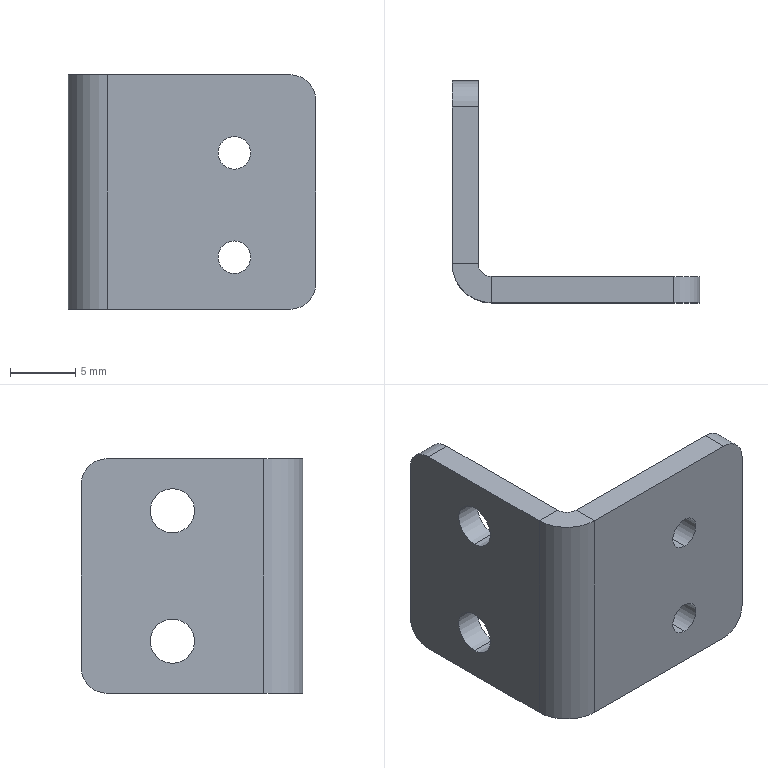Part | NX | features BREP 1 | 1 solid | 26 faces | box 19 x 17 x 18 mm | volume 1130 mm3 | cylinder 14 | plane 12 | commonest cylinder face diameters 2.5 x4 3.4 x4 4 x4 2 x1 6 x1
STEP:
#1=CARTESIAN_POINT('',(-2.,8.,6.7));
#2=VERTEX_POINT('',#1);
#3=CARTESIAN_POINT('',(0.,8.,6.7));
#4=VERTEX_POINT('',#3);
#5=CARTESIAN_POINT('',(0.,8.,6.7));
#6=DIRECTION('',(1.,0.,0.));
#7=VECTOR('',#6,1000.);
#8=LINE('',#5,#7);
#9=EDGE_CURVE('',#2,#4,#8,.T.);
#10=ORIENTED_EDGE('',*,*,#9,.F.);
#11=CARTESIAN_POINT('',(-2.,8.,3.3));
#12=VERTEX_POINT('',#11);
#13=CARTESIAN_POINT('',(-2.,8.,5.));
#14=DIRECTION('',(1.,0.,0.));
#15=DIRECTION('',(0.,0.,-1.));
#16=AXIS2_PLACEMENT_3D('',#13,#14,#15);
#17=CIRCLE('',#16,1.7);
#18=EDGE_CURVE('',#12,#2,#17,.T.);
#19=ORIENTED_EDGE('',*,*,#18,.F.);
#20=CARTESIAN_POINT('',(0.,8.,3.3));
#21=VERTEX_POINT('',#20);
#22=CARTESIAN_POINT('',(0.,8.,3.3));
#23=DIRECTION('',(1.,0.,0.));
#24=VECTOR('',#23,1000.);
#25=LINE('',#22,#24);
#26=EDGE_CURVE('',#12,#21,#25,.T.);
#27=ORIENTED_EDGE('',*,*,#26,.T.);
#28=CARTESIAN_POINT('',(0.,8.,5.));
#29=DIRECTION('',(1.,0.,0.));
#30=DIRECTION('',(0.,0.,-1.));
#31=AXIS2_PLACEMENT_3D('',#28,#29,#30);
#32=CIRCLE('',#31,1.7);
#33=EDGE_CURVE('',#21,#4,#32,.T.);
#34=ORIENTED_EDGE('',*,*,#33,.T.);
#35=EDGE_LOOP('',(#10,#19,#27,#34));
#36=FACE_BOUND('',#35,.T.);
#37=CARTESIAN_POINT('',(0.,8.,5.));
#38=DIRECTION('',(1.,0.,0.));
#39=DIRECTION('',(0.,0.,-1.));
#40=AXIS2_PLACEMENT_3D('',#37,#38,#39);
#41=CYLINDRICAL_SURFACE('',#40,1.7);
#42=ADVANCED_FACE('',(#36),#41,.F.);
#43=CARTESIAN_POINT('',(-2.,8.,-3.3));
#44=VERTEX_POINT('',#43);
#45=CARTESIAN_POINT('',(0.,8.,-3.3));
#46=VERTEX_POINT('',#45);
#47=CARTESIAN_POINT('',(0.,8.,-3.3));
#48=DIRECTION('',(1.,0.,0.));
#49=VECTOR('',#48,1000.);
#50=LINE('',#47,#49);
#51=EDGE_CURVE('',#44,#46,#50,.T.);
#52=ORIENTED_EDGE('',*,*,#51,.F.);
#53=CARTESIAN_POINT('',(-2.,8.,-6.7));
#54=VERTEX_POINT('',#53);
#55=CARTESIAN_POINT('',(-2.,8.,-5.));
#56=DIRECTION('',(1.,0.,0.));
#57=DIRECTION('',(0.,0.,-1.));
#58=AXIS2_PLACEMENT_3D('',#55,#56,#57);
#59=CIRCLE('',#58,1.7);
#60=EDGE_CURVE('',#54,#44,#59,.T.);
#61=ORIENTED_EDGE('',*,*,#60,.F.);
#62=CARTESIAN_POINT('',(0.,8.,-6.7));
#63=VERTEX_POINT('',#62);
#64=CARTESIAN_POINT('',(0.,8.,-6.7));
#65=DIRECTION('',(1.,0.,0.));
#66=VECTOR('',#65,1000.);
#67=LINE('',#64,#66);
#68=EDGE_CURVE('',#54,#63,#67,.T.);
#69=ORIENTED_EDGE('',*,*,#68,.T.);
#70=CARTESIAN_POINT('',(0.,8.,-5.));
#71=DIRECTION('',(1.,0.,0.));
#72=DIRECTION('',(0.,0.,-1.));
#73=AXIS2_PLACEMENT_3D('',#70,#71,#72);
#74=CIRCLE('',#73,1.7);
#75=EDGE_CURVE('',#63,#46,#74,.T.);
#76=ORIENTED_EDGE('',*,*,#75,.T.);
#77=EDGE_LOOP('',(#52,#61,#69,#76));
#78=FACE_BOUND('',#77,.T.);
#79=CARTESIAN_POINT('',(0.,8.,-5.));
#80=DIRECTION('',(1.,0.,0.));
#81=DIRECTION('',(0.,0.,-1.));
#82=AXIS2_PLACEMENT_3D('',#79,#80,#81);
#83=CYLINDRICAL_SURFACE('',#82,1.7);
#84=ADVANCED_FACE('',(#78),#83,.F.);
#85=CARTESIAN_POINT('',(10.75,0.,4.25));
#86=VERTEX_POINT('',#85);
#87=CARTESIAN_POINT('',(10.75,-2.,4.25));
#88=VERTEX_POINT('',#87);
#89=CARTESIAN_POINT('',(10.75,-2.,4.25));
#90=DIRECTION('',(0.,-1.,0.));
#91=VECTOR('',#90,1000.);
#92=LINE('',#89,#91);
#93=EDGE_CURVE('',#86,#88,#92,.T.);
#94=ORIENTED_EDGE('',*,*,#93,.F.);
#95=CARTESIAN_POINT('',(10.75,0.,1.75));
#96=VERTEX_POINT('',#95);
#97=CARTESIAN_POINT('',(10.75,0.,3.));
#98=DIRECTION('',(0.,1.,0.));
#99=DIRECTION('',(0.,0.,1.));
#100=AXIS2_PLACEMENT_3D('',#97,#98,#99);
#101=CIRCLE('',#100,1.25);
#102=EDGE_CURVE('',#86,#96,#101,.T.);
#103=ORIENTED_EDGE('',*,*,#102,.T.);
#104=CARTESIAN_POINT('',(10.75,-2.,1.75));
#105=VERTEX_POINT('',#104);
#106=CARTESIAN_POINT('',(10.75,-2.,1.75));
#107=DIRECTION('',(0.,-1.,0.));
#108=VECTOR('',#107,1000.);
#109=LINE('',#106,#108);
#110=EDGE_CURVE('',#96,#105,#109,.T.);
#111=ORIENTED_EDGE('',*,*,#110,.T.);
#112=CARTESIAN_POINT('',(10.75,-2.,3.));
#113=DIRECTION('',(0.,-1.,0.));
#114=DIRECTION('',(0.,0.,-1.));
#115=AXIS2_PLACEMENT_3D('',#112,#113,#114);
#116=CIRCLE('',#115,1.25);
#117=EDGE_CURVE('',#105,#88,#116,.T.);
#118=ORIENTED_EDGE('',*,*,#117,.T.);
#119=EDGE_LOOP('',(#94,#103,#111,#118));
#120=FACE_BOUND('',#119,.T.);
#121=CARTESIAN_POINT('',(10.75,-2.,3.));
#122=DIRECTION('',(0.,-1.,0.));
#123=DIRECTION('',(0.,0.,-1.));
#124=AXIS2_PLACEMENT_3D('',#121,#122,#123);
#125=CYLINDRICAL_SURFACE('',#124,1.25);
#126=ADVANCED_FACE('',(#120),#125,.F.);
#127=CARTESIAN_POINT('',(10.75,0.,-3.75));
#128=VERTEX_POINT('',#127);
#129=CARTESIAN_POINT('',(10.75,-2.,-3.75));
#130=VERTEX_POINT('',#129);
#131=CARTESIAN_POINT('',(10.75,-2.,-3.75));
#132=DIRECTION('',(0.,-1.,0.));
#133=VECTOR('',#132,1000.);
#134=LINE('',#131,#133);
#135=EDGE_CURVE('',#128,#130,#134,.T.);
#136=ORIENTED_EDGE('',*,*,#135,.F.);
#137=CARTESIAN_POINT('',(10.75,0.,-6.25));
#138=VERTEX_POINT('',#137);
#139=CARTESIAN_POINT('',(10.75,0.,-5.));
#140=DIRECTION('',(0.,1.,0.));
#141=DIRECTION('',(0.,0.,1.));
#142=AXIS2_PLACEMENT_3D('',#139,#140,#141);
#143=CIRCLE('',#142,1.25);
#144=EDGE_CURVE('',#128,#138,#143,.T.);
#145=ORIENTED_EDGE('',*,*,#144,.T.);
#146=CARTESIAN_POINT('',(10.75,-2.,-6.25));
#147=VERTEX_POINT('',#146);
#148=CARTESIAN_POINT('',(10.75,-2.,-6.25));
#149=DIRECTION('',(0.,-1.,0.));
#150=VECTOR('',#149,1000.);
#151=LINE('',#148,#150);
#152=EDGE_CURVE('',#138,#147,#151,.T.);
#153=ORIENTED_EDGE('',*,*,#152,.T.);
#154=CARTESIAN_POINT('',(10.75,-2.,-5.));
#155=DIRECTION('',(0.,-1.,0.));
#156=DIRECTION('',(0.,0.,-1.));
#157=AXIS2_PLACEMENT_3D('',#154,#155,#156);
#158=CIRCLE('',#157,1.25);
#159=EDGE_CURVE('',#147,#130,#158,.T.);
#160=ORIENTED_EDGE('',*,*,#159,.T.);
#161=EDGE_LOOP('',(#136,#145,#153,#160));
#162=FACE_BOUND('',#161,.T.);
#163=CARTESIAN_POINT('',(10.75,-2.,-5.));
#164=DIRECTION('',(0.,-1.,0.));
#165=DIRECTION('',(0.,0.,-1.));
#166=AXIS2_PLACEMENT_3D('',#163,#164,#165);
#167=CYLINDRICAL_SURFACE('',#166,1.25);
#168=ADVANCED_FACE('',(#162),#167,.F.);
#169=CARTESIAN_POINT('',(-2.,15.,-7.));
#170=VERTEX_POINT('',#169);
#171=CARTESIAN_POINT('',(-2.,13.,-9.));
#172=VERTEX_POINT('',#171);
#173=CARTESIAN_POINT('',(-2.,13.,-7.));
#174=DIRECTION('',(-1.,0.,0.));
#175=DIRECTION('',(0.,1.,0.));
#176=AXIS2_PLACEMENT_3D('',#173,#174,#175);
#177=CIRCLE('',#176,2.);
#178=EDGE_CURVE('',#170,#172,#177,.T.);
#179=ORIENTED_EDGE('',*,*,#178,.F.);
#180=CARTESIAN_POINT('',(0.,15.,-7.));
#181=VERTEX_POINT('',#180);
#182=CARTESIAN_POINT('',(-2.,15.,-7.));
#183=DIRECTION('',(-1.,0.,0.));
#184=VECTOR('',#183,1000.);
#185=LINE('',#182,#184);
#186=EDGE_CURVE('',#181,#170,#185,.T.);
#187=ORIENTED_EDGE('',*,*,#186,.F.);
#188=CARTESIAN_POINT('',(0.,13.,-9.));
#189=VERTEX_POINT('',#188);
#190=CARTESIAN_POINT('',(0.,13.,-7.));
#191=DIRECTION('',(1.,0.,0.));
#192=DIRECTION('',(0.,1.,0.));
#193=AXIS2_PLACEMENT_3D('',#190,#191,#192);
#194=CIRCLE('',#193,2.);
#195=EDGE_CURVE('',#189,#181,#194,.T.);
#196=ORIENTED_EDGE('',*,*,#195,.F.);
#197=CARTESIAN_POINT('',(1.,13.,-9.));
#198=DIRECTION('',(1.,0.,0.));
#199=VECTOR('',#198,1000.);
#200=LINE('',#197,#199);
#201=EDGE_CURVE('',#172,#189,#200,.T.);
#202=ORIENTED_EDGE('',*,*,#201,.F.);
#203=EDGE_LOOP('',(#179,#187,#196,#202));
#204=FACE_BOUND('',#203,.T.);
#205=CARTESIAN_POINT('',(1.,13.,-7.));
#206=DIRECTION('',(1.,0.,0.));
#207=DIRECTION('',(0.,0.,-1.));
#208=AXIS2_PLACEMENT_3D('',#205,#206,#207);
#209=CYLINDRICAL_SURFACE('',#208,2.);
#210=ADVANCED_FACE('',(#204),#209,.T.);
#211=CARTESIAN_POINT('',(-2.,13.,9.));
#212=VERTEX_POINT('',#211);
#213=CARTESIAN_POINT('',(-2.,15.,7.));
#214=VERTEX_POINT('',#213);
#215=CARTESIAN_POINT('',(-2.,13.,7.));
#216=DIRECTION('',(-1.,0.,0.));
#217=DIRECTION('',(0.,1.,0.));
#218=AXIS2_PLACEMENT_3D('',#215,#216,#217);
#219=CIRCLE('',#218,2.);
#220=EDGE_CURVE('',#212,#214,#219,.T.);
#221=ORIENTED_EDGE('',*,*,#220,.F.);
#222=CARTESIAN_POINT('',(0.,13.,9.));
#223=VERTEX_POINT('',#222);
#224=CARTESIAN_POINT('',(-2.,13.,9.));
#225=DIRECTION('',(-1.,0.,0.));
#226=VECTOR('',#225,1000.);
#227=LINE('',#224,#226);
#228=EDGE_CURVE('',#223,#212,#227,.T.);
#229=ORIENTED_EDGE('',*,*,#228,.F.);
#230=CARTESIAN_POINT('',(0.,15.,7.));
#231=VERTEX_POINT('',#230);
#232=CARTESIAN_POINT('',(0.,13.,7.));
#233=DIRECTION('',(1.,0.,0.));
#234=DIRECTION('',(0.,1.,0.));
#235=AXIS2_PLACEMENT_3D('',#232,#233,#234);
#236=CIRCLE('',#235,2.);
#237=EDGE_CURVE('',#231,#223,#236,.T.);
#238=ORIENTED_EDGE('',*,*,#237,.F.);
#239=CARTESIAN_POINT('',(0.,15.,7.));
#240=DIRECTION('',(1.,0.,0.));
#241=VECTOR('',#240,1000.);
#242=LINE('',#239,#241);
#243=EDGE_CURVE('',#214,#231,#242,.T.);
#244=ORIENTED_EDGE('',*,*,#243,.F.);
#245=EDGE_LOOP('',(#221,#229,#238,#244));
#246=FACE_BOUND('',#245,.T.);
#247=CARTESIAN_POINT('',(-2.,13.,7.));
#248=DIRECTION('',(-1.,0.,0.));
#249=DIRECTION('',(0.,0.,1.));
#250=AXIS2_PLACEMENT_3D('',#247,#248,#249);
#251=CYLINDRICAL_SURFACE('',#250,2.);
#252=ADVANCED_FACE('',(#246),#251,.T.);
#253=CARTESIAN_POINT('',(15.,0.,9.));
#254=VERTEX_POINT('',#253);
#255=CARTESIAN_POINT('',(17.,0.,7.));
#256=VERTEX_POINT('',#255);
#257=CARTESIAN_POINT('',(15.,0.,7.));
#258=DIRECTION('',(0.,1.,0.));
#259=DIRECTION('',(0.,0.,1.));
#260=AXIS2_PLACEMENT_3D('',#257,#258,#259);
#261=CIRCLE('',#260,2.);
#262=EDGE_CURVE('',#254,#256,#261,.T.);
#263=ORIENTED_EDGE('',*,*,#262,.F.);
#264=CARTESIAN_POINT('',(15.,-2.,9.));
#265=VERTEX_POINT('',#264);
#266=CARTESIAN_POINT('',(15.,1.,9.));
#267=DIRECTION('',(0.,1.,0.));
#268=VECTOR('',#267,1000.);
#269=LINE('',#266,#268);
#270=EDGE_CURVE('',#265,#254,#269,.T.);
#271=ORIENTED_EDGE('',*,*,#270,.F.);
#272=CARTESIAN_POINT('',(17.,-2.,7.));
#273=VERTEX_POINT('',#272);
#274=CARTESIAN_POINT('',(15.,-2.,7.));
#275=DIRECTION('',(0.,-1.,0.));
#276=DIRECTION('',(0.,0.,1.));
#277=AXIS2_PLACEMENT_3D('',#274,#275,#276);
#278=CIRCLE('',#277,2.);
#279=EDGE_CURVE('',#273,#265,#278,.T.);
#280=ORIENTED_EDGE('',*,*,#279,.F.);
#281=CARTESIAN_POINT('',(17.,0.,7.));
#282=DIRECTION('',(0.,-1.,0.));
#283=VECTOR('',#282,1000.);
#284=LINE('',#281,#283);
#285=EDGE_CURVE('',#256,#273,#284,.T.);
#286=ORIENTED_EDGE('',*,*,#285,.F.);
#287=EDGE_LOOP('',(#263,#271,#280,#286));
#288=FACE_BOUND('',#287,.T.);
#289=CARTESIAN_POINT('',(15.,0.,7.));
#290=DIRECTION('',(0.,-1.,0.));
#291=DIRECTION('',(0.,0.,-1.));
#292=AXIS2_PLACEMENT_3D('',#289,#290,#291);
#293=CYLINDRICAL_SURFACE('',#292,2.);
#294=ADVANCED_FACE('',(#288),#293,.T.);
#295=CARTESIAN_POINT('',(17.,0.,-7.));
#296=VERTEX_POINT('',#295);
#297=CARTESIAN_POINT('',(15.,0.,-9.));
#298=VERTEX_POINT('',#297);
#299=CARTESIAN_POINT('',(15.,0.,-7.));
#300=DIRECTION('',(0.,1.,0.));
#301=DIRECTION('',(0.,0.,1.));
#302=AXIS2_PLACEMENT_3D('',#299,#300,#301);
#303=CIRCLE('',#302,2.);
#304=EDGE_CURVE('',#296,#298,#303,.T.);
#305=ORIENTED_EDGE('',*,*,#304,.F.);
#306=CARTESIAN_POINT('',(17.,-2.,-7.));
#307=VERTEX_POINT('',#306);
#308=CARTESIAN_POINT('',(17.,0.,-7.));
#309=DIRECTION('',(0.,1.,0.));
#310=VECTOR('',#309,1000.);
#311=LINE('',#308,#310);
#312=EDGE_CURVE('',#307,#296,#311,.T.);
#313=ORIENTED_EDGE('',*,*,#312,.F.);
#314=CARTESIAN_POINT('',(15.,-2.,-9.));
#315=VERTEX_POINT('',#314);
#316=CARTESIAN_POINT('',(15.,-2.,-7.));
#317=DIRECTION('',(0.,-1.,0.));
#318=DIRECTION('',(0.,0.,1.));
#319=AXIS2_PLACEMENT_3D('',#316,#317,#318);
#320=CIRCLE('',#319,2.);
#321=EDGE_CURVE('',#315,#307,#320,.T.);
#322=ORIENTED_EDGE('',*,*,#321,.F.);
#323=CARTESIAN_POINT('',(15.,1.,-9.));
#324=DIRECTION('',(0.,-1.,0.));
#325=VECTOR('',#324,1000.);
#326=LINE('',#323,#325);
#327=EDGE_CURVE('',#298,#315,#326,.T.);
#328=ORIENTED_EDGE('',*,*,#327,.F.);
#329=EDGE_LOOP('',(#305,#313,#322,#328));
#330=FACE_BOUND('',#329,.T.);
#331=CARTESIAN_POINT('',(15.,1.,-7.));
#332=DIRECTION('',(0.,-1.,0.));
#333=DIRECTION('',(0.,0.,-1.));
#334=AXIS2_PLACEMENT_3D('',#331,#332,#333);
#335=CYLINDRICAL_SURFACE('',#334,2.);
#336=ADVANCED_FACE('',(#330),#335,.T.);
#337=CARTESIAN_POINT('',(1.,0.,-9.));
#338=VERTEX_POINT('',#337);
#339=CARTESIAN_POINT('',(0.,0.,-9.));
#340=DIRECTION('',(1.,0.,0.));
#341=VECTOR('',#340,1000.);
#342=LINE('',#339,#341);
#343=EDGE_CURVE('',#338,#298,#342,.T.);
#344=ORIENTED_EDGE('',*,*,#343,.T.);
#345=ORIENTED_EDGE('',*,*,#327,.T.);
#346=CARTESIAN_POINT('',(1.,-2.,-9.));
#347=VERTEX_POINT('',#346);
#348=CARTESIAN_POINT('',(0.,-2.,-9.));
#349=DIRECTION('',(1.,0.,0.));
#350=VECTOR('',#349,1000.);
#351=LINE('',#348,#350);
#352=EDGE_CURVE('',#347,#315,#351,.T.);
#353=ORIENTED_EDGE('',*,*,#352,.F.);
#354=CARTESIAN_POINT('',(1.,-2.,-9.));
#355=DIRECTION('',(0.,1.,0.));
#356=VECTOR('',#355,1000.);
#357=LINE('',#354,#356);
#358=EDGE_CURVE('',#347,#338,#357,.T.);
#359=ORIENTED_EDGE('',*,*,#358,.T.);
#360=EDGE_LOOP('',(#344,#345,#353,#359));
#361=FACE_BOUND('',#360,.T.);
#362=CARTESIAN_POINT('',(1.,1.,-9.));
#363=DIRECTION('',(0.,0.,-1.));
#364=DIRECTION('',(-1.,0.,0.));
#365=AXIS2_PLACEMENT_3D('',#362,#363,#364);
#366=PLANE('',#365);
#367=ADVANCED_FACE('',(#361),#366,.T.);
#368=CARTESIAN_POINT('',(0.,1.,9.));
#369=VERTEX_POINT('',#368);
#370=CARTESIAN_POINT('',(0.,15.,9.));
#371=DIRECTION('',(0.,-1.,0.));
#372=VECTOR('',#371,1000.);
#373=LINE('',#370,#372);
#374=EDGE_CURVE('',#223,#369,#373,.T.);
#375=ORIENTED_EDGE('',*,*,#374,.F.);
#376=ORIENTED_EDGE('',*,*,#228,.T.);
#377=CARTESIAN_POINT('',(-2.,1.,9.));
#378=VERTEX_POINT('',#377);
#379=CARTESIAN_POINT('',(-2.,15.,9.));
#380=DIRECTION('',(0.,-1.,0.));
#381=VECTOR('',#380,1000.);
#382=LINE('',#379,#381);
#383=EDGE_CURVE('',#212,#378,#382,.T.);
#384=ORIENTED_EDGE('',*,*,#383,.T.);
#385=CARTESIAN_POINT('',(-2.,1.,9.));
#386=DIRECTION('',(1.,0.,0.));
#387=VECTOR('',#386,1000.);
#388=LINE('',#385,#387);
#389=EDGE_CURVE('',#378,#369,#388,.T.);
#390=ORIENTED_EDGE('',*,*,#389,.T.);
#391=EDGE_LOOP('',(#375,#376,#384,#390));
#392=FACE_BOUND('',#391,.T.);
#393=CARTESIAN_POINT('',(1.,1.,9.));
#394=DIRECTION('',(0.,0.,-1.));
#395=DIRECTION('',(-1.,0.,0.));
#396=AXIS2_PLACEMENT_3D('',#393,#394,#395);
#397=PLANE('',#396);
#398=ADVANCED_FACE('',(#392),#397,.F.);
#399=CARTESIAN_POINT('',(-2.,1.,-9.));
#400=VERTEX_POINT('',#399);
#401=CARTESIAN_POINT('',(1.,1.,-9.));
#402=DIRECTION('',(0.,0.,1.));
#403=DIRECTION('',(1.,0.,0.));
#404=AXIS2_PLACEMENT_3D('',#401,#402,#403);
#405=CIRCLE('',#404,3.);
#406=EDGE_CURVE('',#400,#347,#405,.T.);
#407=ORIENTED_EDGE('',*,*,#406,.T.);
#408=CARTESIAN_POINT('',(1.,-2.,9.));
#409=VERTEX_POINT('',#408);
#410=CARTESIAN_POINT('',(1.,-2.,9.));
#411=DIRECTION('',(0.,0.,-1.));
#412=VECTOR('',#411,1000.);
#413=LINE('',#410,#412);
#414=EDGE_CURVE('',#409,#347,#413,.T.);
#415=ORIENTED_EDGE('',*,*,#414,.F.);
#416=CARTESIAN_POINT('',(1.,1.,9.));
#417=DIRECTION('',(0.,0.,1.));
#418=DIRECTION('',(1.,0.,0.));
#419=AXIS2_PLACEMENT_3D('',#416,#417,#418);
#420=CIRCLE('',#419,3.);
#421=EDGE_CURVE('',#378,#409,#420,.T.);
#422=ORIENTED_EDGE('',*,*,#421,.F.);
#423=CARTESIAN_POINT('',(-2.,1.,9.));
#424=DIRECTION('',(0.,0.,-1.));
#425=VECTOR('',#424,1000.);
#426=LINE('',#423,#425);
#427=EDGE_CURVE('',#378,#400,#426,.T.);
#428=ORIENTED_EDGE('',*,*,#427,.T.);
#429=EDGE_LOOP('',(#407,#415,#422,#428));
#430=FACE_BOUND('',#429,.T.);
#431=CARTESIAN_POINT('',(1.,1.,9.));
#432=DIRECTION('',(0.,0.,-1.));
#433=DIRECTION('',(-1.,0.,0.));
#434=AXIS2_PLACEMENT_3D('',#431,#432,#433);
#435=CYLINDRICAL_SURFACE('',#434,3.);
#436=ADVANCED_FACE('',(#430),#435,.T.);
#437=ORIENTED_EDGE('',*,*,#383,.F.);
#438=ORIENTED_EDGE('',*,*,#220,.T.);
#439=CARTESIAN_POINT('',(-2.,15.,9.));
#440=DIRECTION('',(0.,0.,-1.));
#441=VECTOR('',#440,1000.);
#442=LINE('',#439,#441);
#443=EDGE_CURVE('',#214,#170,#442,.T.);
#444=ORIENTED_EDGE('',*,*,#443,.T.);
#445=ORIENTED_EDGE('',*,*,#178,.T.);
#446=CARTESIAN_POINT('',(-2.,15.,-9.));
#447=DIRECTION('',(0.,-1.,0.));
#448=VECTOR('',#447,1000.);
#449=LINE('',#446,#448);
#450=EDGE_CURVE('',#172,#400,#449,.T.);
#451=ORIENTED_EDGE('',*,*,#450,.T.);
#452=ORIENTED_EDGE('',*,*,#427,.F.);
#453=EDGE_LOOP('',(#437,#438,#444,#445,#451,#452));
#454=FACE_BOUND('',#453,.T.);
#455=ORIENTED_EDGE('',*,*,#60,.T.);
#456=CARTESIAN_POINT('',(-2.,8.,-5.));
#457=DIRECTION('',(1.,0.,0.));
#458=DIRECTION('',(0.,0.,-1.));
#459=AXIS2_PLACEMENT_3D('',#456,#457,#458);
#460=CIRCLE('',#459,1.7);
#461=EDGE_CURVE('',#44,#54,#460,.T.);
#462=ORIENTED_EDGE('',*,*,#461,.T.);
#463=EDGE_LOOP('',(#455,#462));
#464=FACE_BOUND('',#463,.T.);
#465=ORIENTED_EDGE('',*,*,#18,.T.);
#466=CARTESIAN_POINT('',(-2.,8.,5.));
#467=DIRECTION('',(1.,0.,0.));
#468=DIRECTION('',(0.,0.,-1.));
#469=AXIS2_PLACEMENT_3D('',#466,#467,#468);
#470=CIRCLE('',#469,1.7);
#471=EDGE_CURVE('',#2,#12,#470,.T.);
#472=ORIENTED_EDGE('',*,*,#471,.T.);
#473=EDGE_LOOP('',(#465,#472));
#474=FACE_BOUND('',#473,.T.);
#475=CARTESIAN_POINT('',(-2.,15.,9.));
#476=DIRECTION('',(1.,0.,0.));
#477=DIRECTION('',(0.,1.,0.));
#478=AXIS2_PLACEMENT_3D('',#475,#476,#477);
#479=PLANE('',#478);
#480=ADVANCED_FACE('',(#454,#464,#474),#479,.F.);
#481=ORIENTED_EDGE('',*,*,#443,.F.);
#482=ORIENTED_EDGE('',*,*,#243,.T.);
#483=CARTESIAN_POINT('',(0.,15.,9.));
#484=DIRECTION('',(0.,0.,-1.));
#485=VECTOR('',#484,1000.);
#486=LINE('',#483,#485);
#487=EDGE_CURVE('',#231,#181,#486,.T.);
#488=ORIENTED_EDGE('',*,*,#487,.T.);
#489=ORIENTED_EDGE('',*,*,#186,.T.);
#490=EDGE_LOOP('',(#481,#482,#488,#489));
#491=FACE_BOUND('',#490,.T.);
#492=CARTESIAN_POINT('',(-2.,15.,9.));
#493=DIRECTION('',(0.,1.,0.));
#494=DIRECTION('',(0.,0.,1.));
#495=AXIS2_PLACEMENT_3D('',#492,#493,#494);
#496=PLANE('',#495);
#497=ADVANCED_FACE('',(#491),#496,.T.);
#498=ORIENTED_EDGE('',*,*,#487,.F.);
#499=ORIENTED_EDGE('',*,*,#237,.T.);
#500=ORIENTED_EDGE('',*,*,#374,.T.);
#501=CARTESIAN_POINT('',(0.,1.,-9.));
#502=VERTEX_POINT('',#501);
#503=CARTESIAN_POINT('',(0.,1.,9.));
#504=DIRECTION('',(0.,0.,-1.));
#505=VECTOR('',#504,1000.);
#506=LINE('',#503,#505);
#507=EDGE_CURVE('',#369,#502,#506,.T.);
#508=ORIENTED_EDGE('',*,*,#507,.T.);
#509=CARTESIAN_POINT('',(0.,15.,-9.));
#510=DIRECTION('',(0.,-1.,0.));
#511=VECTOR('',#510,1000.);
#512=LINE('',#509,#511);
#513=EDGE_CURVE('',#189,#502,#512,.T.);
#514=ORIENTED_EDGE('',*,*,#513,.F.);
#515=ORIENTED_EDGE('',*,*,#195,.T.);
#516=EDGE_LOOP('',(#498,#499,#500,#508,#514,#515));
#517=FACE_BOUND('',#516,.T.);
#518=ORIENTED_EDGE('',*,*,#75,.F.);
#519=CARTESIAN_POINT('',(0.,8.,-5.));
#520=DIRECTION('',(1.,0.,0.));
#521=DIRECTION('',(0.,0.,-1.));
#522=AXIS2_PLACEMENT_3D('',#519,#520,#521);
#523=CIRCLE('',#522,1.7);
#524=EDGE_CURVE('',#46,#63,#523,.T.);
#525=ORIENTED_EDGE('',*,*,#524,.F.);
#526=EDGE_LOOP('',(#518,#525));
#527=FACE_BOUND('',#526,.T.);
#528=ORIENTED_EDGE('',*,*,#33,.F.);
#529=CARTESIAN_POINT('',(0.,8.,5.));
#530=DIRECTION('',(1.,0.,0.));
#531=DIRECTION('',(0.,0.,-1.));
#532=AXIS2_PLACEMENT_3D('',#529,#530,#531);
#533=CIRCLE('',#532,1.7);
#534=EDGE_CURVE('',#4,#21,#533,.T.);
#535=ORIENTED_EDGE('',*,*,#534,.F.);
#536=EDGE_LOOP('',(#528,#535));
#537=FACE_BOUND('',#536,.T.);
#538=CARTESIAN_POINT('',(0.,15.,9.));
#539=DIRECTION('',(1.,0.,0.));
#540=DIRECTION('',(0.,1.,0.));
#541=AXIS2_PLACEMENT_3D('',#538,#539,#540);
#542=PLANE('',#541);
#543=ADVANCED_FACE('',(#517,#527,#537),#542,.T.);
#544=CARTESIAN_POINT('',(1.,1.,-9.));
#545=DIRECTION('',(0.,0.,1.));
#546=DIRECTION('',(-1.,0.,0.));
#547=AXIS2_PLACEMENT_3D('',#544,#545,#546);
#548=CIRCLE('',#547,1.);
#549=EDGE_CURVE('',#502,#338,#548,.T.);
#550=ORIENTED_EDGE('',*,*,#549,.F.);
#551=ORIENTED_EDGE('',*,*,#507,.F.);
#552=CARTESIAN_POINT('',(1.,0.,9.));
#553=VERTEX_POINT('',#552);
#554=CARTESIAN_POINT('',(1.,1.,9.));
#555=DIRECTION('',(0.,0.,1.));
#556=DIRECTION('',(-1.,0.,0.));
#557=AXIS2_PLACEMENT_3D('',#554,#555,#556);
#558=CIRCLE('',#557,1.);
#559=EDGE_CURVE('',#369,#553,#558,.T.);
#560=ORIENTED_EDGE('',*,*,#559,.T.);
#561=CARTESIAN_POINT('',(1.,0.,9.));
#562=DIRECTION('',(0.,0.,-1.));
#563=VECTOR('',#562,1000.);
#564=LINE('',#561,#563);
#565=EDGE_CURVE('',#553,#338,#564,.T.);
#566=ORIENTED_EDGE('',*,*,#565,.T.);
#567=EDGE_LOOP('',(#550,#551,#560,#566));
#568=FACE_BOUND('',#567,.T.);
#569=CARTESIAN_POINT('',(1.,1.,9.));
#570=DIRECTION('',(0.,0.,-1.));
#571=DIRECTION('',(-1.,0.,0.));
#572=AXIS2_PLACEMENT_3D('',#569,#570,#571);
#573=CYLINDRICAL_SURFACE('',#572,1.);
#574=ADVANCED_FACE('',(#568),#573,.F.);
#575=CARTESIAN_POINT('',(17.,0.,9.));
#576=DIRECTION('',(0.,0.,-1.));
#577=VECTOR('',#576,1000.);
#578=LINE('',#575,#577);
#579=EDGE_CURVE('',#256,#296,#578,.T.);
#580=ORIENTED_EDGE('',*,*,#579,.T.);
#581=ORIENTED_EDGE('',*,*,#304,.T.);
#582=ORIENTED_EDGE('',*,*,#343,.F.);
#583=ORIENTED_EDGE('',*,*,#565,.F.);
#584=CARTESIAN_POINT('',(0.,0.,9.));
#585=DIRECTION('',(1.,0.,0.));
#586=VECTOR('',#585,1000.);
#587=LINE('',#584,#586);
#588=EDGE_CURVE('',#553,#254,#587,.T.);
#589=ORIENTED_EDGE('',*,*,#588,.T.);
#590=ORIENTED_EDGE('',*,*,#262,.T.);
#591=EDGE_LOOP('',(#580,#581,#582,#583,#589,#590));
#592=FACE_BOUND('',#591,.T.);
#593=CARTESIAN_POINT('',(10.75,0.,-5.));
#594=DIRECTION('',(0.,1.,0.));
#595=DIRECTION('',(0.,0.,1.));
#596=AXIS2_PLACEMENT_3D('',#593,#594,#595);
#597=CIRCLE('',#596,1.25);
#598=EDGE_CURVE('',#138,#128,#597,.T.);
#599=ORIENTED_EDGE('',*,*,#598,.F.);
#600=ORIENTED_EDGE('',*,*,#144,.F.);
#601=EDGE_LOOP('',(#599,#600));
#602=FACE_BOUND('',#601,.T.);
#603=CARTESIAN_POINT('',(10.75,0.,3.));
#604=DIRECTION('',(0.,1.,0.));
#605=DIRECTION('',(0.,0.,1.));
#606=AXIS2_PLACEMENT_3D('',#603,#604,#605);
#607=CIRCLE('',#606,1.25);
#608=EDGE_CURVE('',#96,#86,#607,.T.);
#609=ORIENTED_EDGE('',*,*,#608,.F.);
#610=ORIENTED_EDGE('',*,*,#102,.F.);
#611=EDGE_LOOP('',(#609,#610));
#612=FACE_BOUND('',#611,.T.);
#613=CARTESIAN_POINT('',(0.,0.,9.));
#614=DIRECTION('',(0.,1.,0.));
#615=DIRECTION('',(0.,0.,1.));
#616=AXIS2_PLACEMENT_3D('',#613,#614,#615);
#617=PLANE('',#616);
#618=ADVANCED_FACE('',(#592,#602,#612),#617,.T.);
#619=CARTESIAN_POINT('',(17.,-2.,9.));
#620=DIRECTION('',(0.,0.,-1.));
#621=VECTOR('',#620,1000.);
#622=LINE('',#619,#621);
#623=EDGE_CURVE('',#273,#307,#622,.T.);
#624=ORIENTED_EDGE('',*,*,#623,.T.);
#625=ORIENTED_EDGE('',*,*,#312,.T.);
#626=ORIENTED_EDGE('',*,*,#579,.F.);
#627=ORIENTED_EDGE('',*,*,#285,.T.);
#628=EDGE_LOOP('',(#624,#625,#626,#627));
#629=FACE_BOUND('',#628,.T.);
#630=CARTESIAN_POINT('',(17.,0.,9.));
#631=DIRECTION('',(1.,0.,0.));
#632=DIRECTION('',(0.,0.,-1.));
#633=AXIS2_PLACEMENT_3D('',#630,#631,#632);
#634=PLANE('',#633);
#635=ADVANCED_FACE('',(#629),#634,.T.);
#636=ORIENTED_EDGE('',*,*,#352,.T.);
#637=ORIENTED_EDGE('',*,*,#321,.T.);
#638=ORIENTED_EDGE('',*,*,#623,.F.);
#639=ORIENTED_EDGE('',*,*,#279,.T.);
#640=CARTESIAN_POINT('',(0.,-2.,9.));
#641=DIRECTION('',(1.,0.,0.));
#642=VECTOR('',#641,1000.);
#643=LINE('',#640,#642);
#644=EDGE_CURVE('',#409,#265,#643,.T.);
#645=ORIENTED_EDGE('',*,*,#644,.F.);
#646=ORIENTED_EDGE('',*,*,#414,.T.);
#647=EDGE_LOOP('',(#636,#637,#638,#639,#645,#646));
#648=FACE_BOUND('',#647,.T.);
#649=ORIENTED_EDGE('',*,*,#159,.F.);
#650=CARTESIAN_POINT('',(10.75,-2.,-5.));
#651=DIRECTION('',(0.,-1.,0.));
#652=DIRECTION('',(0.,0.,-1.));
#653=AXIS2_PLACEMENT_3D('',#650,#651,#652);
#654=CIRCLE('',#653,1.25);
#655=EDGE_CURVE('',#130,#147,#654,.T.);
#656=ORIENTED_EDGE('',*,*,#655,.F.);
#657=EDGE_LOOP('',(#649,#656));
#658=FACE_BOUND('',#657,.T.);
#659=ORIENTED_EDGE('',*,*,#117,.F.);
#660=CARTESIAN_POINT('',(10.75,-2.,3.));
#661=DIRECTION('',(0.,-1.,0.));
#662=DIRECTION('',(0.,0.,-1.));
#663=AXIS2_PLACEMENT_3D('',#660,#661,#662);
#664=CIRCLE('',#663,1.25);
#665=EDGE_CURVE('',#88,#105,#664,.T.);
#666=ORIENTED_EDGE('',*,*,#665,.F.);
#667=EDGE_LOOP('',(#659,#666));
#668=FACE_BOUND('',#667,.T.);
#669=CARTESIAN_POINT('',(0.,-2.,9.));
#670=DIRECTION('',(0.,1.,0.));
#671=DIRECTION('',(0.,0.,1.));
#672=AXIS2_PLACEMENT_3D('',#669,#670,#671);
#673=PLANE('',#672);
#674=ADVANCED_FACE('',(#648,#658,#668),#673,.F.);
#675=ORIENTED_EDGE('',*,*,#450,.F.);
#676=ORIENTED_EDGE('',*,*,#201,.T.);
#677=ORIENTED_EDGE('',*,*,#513,.T.);
#678=CARTESIAN_POINT('',(0.,1.,-9.));
#679=DIRECTION('',(-1.,0.,0.));
#680=VECTOR('',#679,1000.);
#681=LINE('',#678,#680);
#682=EDGE_CURVE('',#502,#400,#681,.T.);
#683=ORIENTED_EDGE('',*,*,#682,.T.);
#684=EDGE_LOOP('',(#675,#676,#677,#683));
#685=FACE_BOUND('',#684,.T.);
#686=CARTESIAN_POINT('',(1.,-2.,-9.));
#687=DIRECTION('',(0.,0.,-1.));
#688=DIRECTION('',(-1.,0.,0.));
#689=AXIS2_PLACEMENT_3D('',#686,#687,#688);
#690=PLANE('',#689);
#691=ADVANCED_FACE('',(#685),#690,.T.);
#692=ORIENTED_EDGE('',*,*,#682,.F.);
#693=ORIENTED_EDGE('',*,*,#549,.T.);
#694=ORIENTED_EDGE('',*,*,#358,.F.);
#695=ORIENTED_EDGE('',*,*,#406,.F.);
#696=EDGE_LOOP('',(#692,#693,#694,#695));
#697=FACE_BOUND('',#696,.T.);
#698=CARTESIAN_POINT('',(0.,1.,-9.));
#699=DIRECTION('',(0.,0.,-1.));
#700=DIRECTION('',(-1.,0.,0.));
#701=AXIS2_PLACEMENT_3D('',#698,#699,#700);
#702=PLANE('',#701);
#703=ADVANCED_FACE('',(#697),#702,.T.);
#704=ORIENTED_EDGE('',*,*,#644,.T.);
#705=ORIENTED_EDGE('',*,*,#270,.T.);
#706=ORIENTED_EDGE('',*,*,#588,.F.);
#707=CARTESIAN_POINT('',(1.,0.,9.));
#708=DIRECTION('',(0.,-1.,0.));
#709=VECTOR('',#708,1000.);
#710=LINE('',#707,#709);
#711=EDGE_CURVE('',#553,#409,#710,.T.);
#712=ORIENTED_EDGE('',*,*,#711,.T.);
#713=EDGE_LOOP('',(#704,#705,#706,#712));
#714=FACE_BOUND('',#713,.T.);
#715=CARTESIAN_POINT('',(-2.,1.,9.));
#716=DIRECTION('',(0.,0.,1.));
#717=DIRECTION('',(1.,0.,0.));
#718=AXIS2_PLACEMENT_3D('',#715,#716,#717);
#719=PLANE('',#718);
#720=ADVANCED_FACE('',(#714),#719,.T.);
#721=ORIENTED_EDGE('',*,*,#711,.F.);
#722=ORIENTED_EDGE('',*,*,#559,.F.);
#723=ORIENTED_EDGE('',*,*,#389,.F.);
#724=ORIENTED_EDGE('',*,*,#421,.T.);
#725=EDGE_LOOP('',(#721,#722,#723,#724));
#726=FACE_BOUND('',#725,.T.);
#727=CARTESIAN_POINT('',(1.,0.,9.));
#728=DIRECTION('',(0.,0.,1.));
#729=DIRECTION('',(1.,0.,0.));
#730=AXIS2_PLACEMENT_3D('',#727,#728,#729);
#731=PLANE('',#730);
#732=ADVANCED_FACE('',(#726),#731,.T.);
#733=ORIENTED_EDGE('',*,*,#598,.T.);
#734=ORIENTED_EDGE('',*,*,#135,.T.);
#735=ORIENTED_EDGE('',*,*,#655,.T.);
#736=ORIENTED_EDGE('',*,*,#152,.F.);
#737=EDGE_LOOP('',(#733,#734,#735,#736));
#738=FACE_BOUND('',#737,.T.);
#739=CARTESIAN_POINT('',(10.75,-2.,-5.));
#740=DIRECTION('',(0.,-1.,0.));
#741=DIRECTION('',(0.,0.,-1.));
#742=AXIS2_PLACEMENT_3D('',#739,#740,#741);
#743=CYLINDRICAL_SURFACE('',#742,1.25);
#744=ADVANCED_FACE('',(#738),#743,.F.);
#745=ORIENTED_EDGE('',*,*,#608,.T.);
#746=ORIENTED_EDGE('',*,*,#93,.T.);
#747=ORIENTED_EDGE('',*,*,#665,.T.);
#748=ORIENTED_EDGE('',*,*,#110,.F.);
#749=EDGE_LOOP('',(#745,#746,#747,#748));
#750=FACE_BOUND('',#749,.T.);
#751=CARTESIAN_POINT('',(10.75,-2.,3.));
#752=DIRECTION('',(0.,-1.,0.));
#753=DIRECTION('',(0.,0.,-1.));
#754=AXIS2_PLACEMENT_3D('',#751,#752,#753);
#755=CYLINDRICAL_SURFACE('',#754,1.25);
#756=ADVANCED_FACE('',(#750),#755,.F.);
#757=ORIENTED_EDGE('',*,*,#461,.F.);
#758=ORIENTED_EDGE('',*,*,#51,.T.);
#759=ORIENTED_EDGE('',*,*,#524,.T.);
#760=ORIENTED_EDGE('',*,*,#68,.F.);
#761=EDGE_LOOP('',(#757,#758,#759,#760));
#762=FACE_BOUND('',#761,.T.);
#763=CARTESIAN_POINT('',(0.,8.,-5.));
#764=DIRECTION('',(1.,0.,0.));
#765=DIRECTION('',(0.,0.,-1.));
#766=AXIS2_PLACEMENT_3D('',#763,#764,#765);
#767=CYLINDRICAL_SURFACE('',#766,1.7);
#768=ADVANCED_FACE('',(#762),#767,.F.);
#769=ORIENTED_EDGE('',*,*,#471,.F.);
#770=ORIENTED_EDGE('',*,*,#9,.T.);
#771=ORIENTED_EDGE('',*,*,#534,.T.);
#772=ORIENTED_EDGE('',*,*,#26,.F.);
#773=EDGE_LOOP('',(#769,#770,#771,#772));
#774=FACE_BOUND('',#773,.T.);
#775=CARTESIAN_POINT('',(0.,8.,5.));
#776=DIRECTION('',(1.,0.,0.));
#777=DIRECTION('',(0.,0.,-1.));
#778=AXIS2_PLACEMENT_3D('',#775,#776,#777);
#779=CYLINDRICAL_SURFACE('',#778,1.7);
#780=ADVANCED_FACE('',(#774),#779,.F.);
#781=CLOSED_SHELL('',(#42,#84,#126,#168,#210,#252,#294,#336,#367,#398,#436,#480,#497,#543,#574,#618,#635,#674,#691,#703,#720,#732,#744,#756,#768,#780));
#782=MANIFOLD_SOLID_BREP('',#781);
#783=(LENGTH_UNIT()NAMED_UNIT(*)SI_UNIT(.MILLI.,.METRE.));
#784=UNCERTAINTY_MEASURE_WITH_UNIT(LENGTH_MEASURE(0.00001),#783,'','');
#785=(NAMED_UNIT(*)PLANE_ANGLE_UNIT()SI_UNIT($,.RADIAN.));
#786=(NAMED_UNIT(*)SI_UNIT($,.STERADIAN.)SOLID_ANGLE_UNIT());
#787=(GEOMETRIC_REPRESENTATION_CONTEXT(3)GLOBAL_UNCERTAINTY_ASSIGNED_CONTEXT((#784))GLOBAL_UNIT_ASSIGNED_CONTEXT((#783,#785,#786))REPRESENTATION_CONTEXT('',''));
#788=ADVANCED_BREP_SHAPE_REPRESENTATION('',(#782),#787);